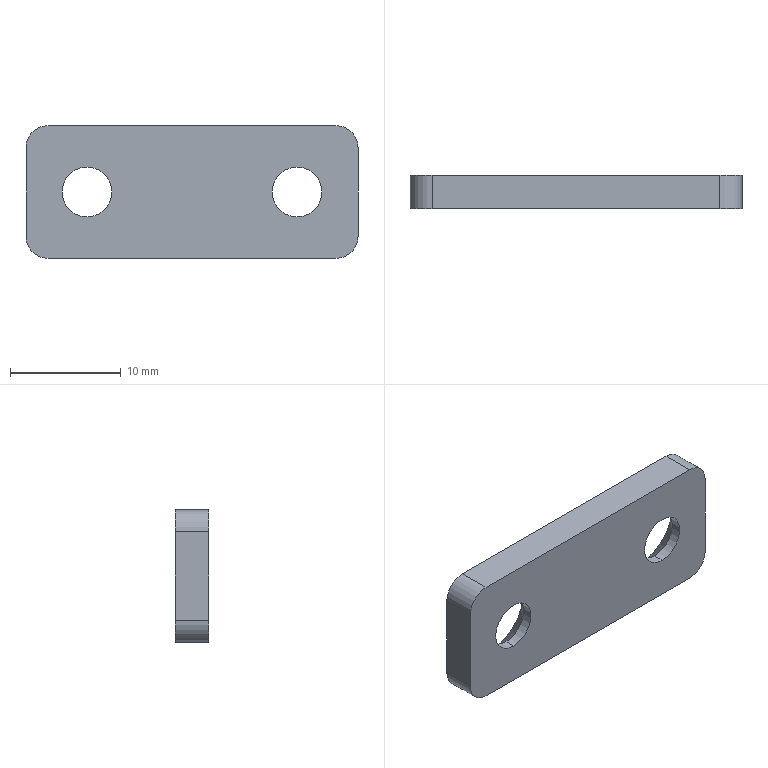Part | STEP file | 03-04 cutter pad block press plate | 1 solid | 18 faces | box 30 x 3 x 12 mm | volume 896.818 mm3 | cylinder 8 | plane 6 | cone 4 | commonest cylinder face diameters 4 x4 4.5 x4
STEP:
#1=CARTESIAN_POINT('',(-9.496,0.95,-2.25));
#2=VERTEX_POINT('',#1);
#3=CARTESIAN_POINT('',(-9.496,0.95,2.25));
#4=VERTEX_POINT('',#3);
#5=CARTESIAN_POINT('',(-9.496,0.95,0.));
#6=DIRECTION('',(0.,1.,0.));
#7=DIRECTION('',(0.,0.,1.));
#8=AXIS2_PLACEMENT_3D('',#5,#6,#7);
#9=CIRCLE('',#8,2.25);
#10=EDGE_CURVE('',#2,#4,#9,.T.);
#11=ORIENTED_EDGE('',*,*,#10,.F.);
#12=CARTESIAN_POINT('',(-9.496,3.,-4.3));
#13=VERTEX_POINT('',#12);
#14=CARTESIAN_POINT('',(-9.496,3.,-4.3));
#15=DIRECTION('',(0.,0.7071,-0.7071));
#16=VECTOR('',#15,1000.);
#17=LINE('',#14,#16);
#18=EDGE_CURVE('',#2,#13,#17,.T.);
#19=ORIENTED_EDGE('',*,*,#18,.T.);
#20=CARTESIAN_POINT('',(-9.496,3.,4.3));
#21=VERTEX_POINT('',#20);
#22=CARTESIAN_POINT('',(-9.496,3.,0.));
#23=DIRECTION('',(0.,1.,0.));
#24=DIRECTION('',(0.,0.,1.));
#25=AXIS2_PLACEMENT_3D('',#22,#23,#24);
#26=CIRCLE('',#25,4.3);
#27=EDGE_CURVE('',#13,#21,#26,.T.);
#28=ORIENTED_EDGE('',*,*,#27,.T.);
#29=CARTESIAN_POINT('',(-9.496,3.,4.3));
#30=DIRECTION('',(0.,0.7071,0.7071));
#31=VECTOR('',#30,1000.);
#32=LINE('',#29,#31);
#33=EDGE_CURVE('',#4,#21,#32,.T.);
#34=ORIENTED_EDGE('',*,*,#33,.F.);
#35=EDGE_LOOP('',(#11,#19,#28,#34));
#36=FACE_OUTER_BOUND('',#35,.T.);
#37=CARTESIAN_POINT('',(-9.496,3.,0.));
#38=DIRECTION('',(0.,1.,0.));
#39=DIRECTION('',(0.,0.,1.));
#40=AXIS2_PLACEMENT_3D('',#37,#38,#39);
#41=CONICAL_SURFACE('',#40,4.3,0.7854);
#42=ADVANCED_FACE('',(#36),#41,.F.);
#43=CARTESIAN_POINT('',(-9.496,0.,-2.25));
#44=VERTEX_POINT('',#43);
#45=CARTESIAN_POINT('',(-9.496,0.,2.25));
#46=VERTEX_POINT('',#45);
#47=CARTESIAN_POINT('',(-9.496,0.,0.));
#48=DIRECTION('',(0.,1.,0.));
#49=DIRECTION('',(0.,0.,1.));
#50=AXIS2_PLACEMENT_3D('',#47,#48,#49);
#51=CIRCLE('',#50,2.25);
#52=EDGE_CURVE('',#44,#46,#51,.T.);
#53=ORIENTED_EDGE('',*,*,#52,.F.);
#54=CARTESIAN_POINT('',(-9.496,3.,-2.25));
#55=DIRECTION('',(0.,1.,0.));
#56=VECTOR('',#55,1000.);
#57=LINE('',#54,#56);
#58=EDGE_CURVE('',#44,#2,#57,.T.);
#59=ORIENTED_EDGE('',*,*,#58,.T.);
#60=ORIENTED_EDGE('',*,*,#10,.T.);
#61=CARTESIAN_POINT('',(-9.496,3.,2.25));
#62=DIRECTION('',(0.,1.,0.));
#63=VECTOR('',#62,1000.);
#64=LINE('',#61,#63);
#65=EDGE_CURVE('',#46,#4,#64,.T.);
#66=ORIENTED_EDGE('',*,*,#65,.F.);
#67=EDGE_LOOP('',(#53,#59,#60,#66));
#68=FACE_OUTER_BOUND('',#67,.T.);
#69=CARTESIAN_POINT('',(-9.496,3.,0.));
#70=DIRECTION('',(0.,1.,0.));
#71=DIRECTION('',(0.,0.,1.));
#72=AXIS2_PLACEMENT_3D('',#69,#70,#71);
#73=CYLINDRICAL_SURFACE('',#72,2.25);
#74=ADVANCED_FACE('',(#68),#73,.F.);
#75=CARTESIAN_POINT('',(9.5,0.95,-2.25));
#76=VERTEX_POINT('',#75);
#77=CARTESIAN_POINT('',(9.5,0.95,2.25));
#78=VERTEX_POINT('',#77);
#79=CARTESIAN_POINT('',(9.5,0.95,0.));
#80=DIRECTION('',(0.,1.,0.));
#81=DIRECTION('',(0.,0.,1.));
#82=AXIS2_PLACEMENT_3D('',#79,#80,#81);
#83=CIRCLE('',#82,2.25);
#84=EDGE_CURVE('',#76,#78,#83,.T.);
#85=ORIENTED_EDGE('',*,*,#84,.F.);
#86=CARTESIAN_POINT('',(9.5,3.,-4.3));
#87=VERTEX_POINT('',#86);
#88=CARTESIAN_POINT('',(9.5,3.,-4.3));
#89=DIRECTION('',(0.,0.7071,-0.7071));
#90=VECTOR('',#89,1000.);
#91=LINE('',#88,#90);
#92=EDGE_CURVE('',#76,#87,#91,.T.);
#93=ORIENTED_EDGE('',*,*,#92,.T.);
#94=CARTESIAN_POINT('',(9.5,3.,4.3));
#95=VERTEX_POINT('',#94);
#96=CARTESIAN_POINT('',(9.5,3.,0.));
#97=DIRECTION('',(0.,1.,0.));
#98=DIRECTION('',(0.,0.,1.));
#99=AXIS2_PLACEMENT_3D('',#96,#97,#98);
#100=CIRCLE('',#99,4.3);
#101=EDGE_CURVE('',#87,#95,#100,.T.);
#102=ORIENTED_EDGE('',*,*,#101,.T.);
#103=CARTESIAN_POINT('',(9.5,3.,4.3));
#104=DIRECTION('',(0.,0.7071,0.7071));
#105=VECTOR('',#104,1000.);
#106=LINE('',#103,#105);
#107=EDGE_CURVE('',#78,#95,#106,.T.);
#108=ORIENTED_EDGE('',*,*,#107,.F.);
#109=EDGE_LOOP('',(#85,#93,#102,#108));
#110=FACE_OUTER_BOUND('',#109,.T.);
#111=CARTESIAN_POINT('',(9.5,3.,0.));
#112=DIRECTION('',(0.,1.,0.));
#113=DIRECTION('',(0.,0.,1.));
#114=AXIS2_PLACEMENT_3D('',#111,#112,#113);
#115=CONICAL_SURFACE('',#114,4.3,0.7854);
#116=ADVANCED_FACE('',(#110),#115,.F.);
#117=CARTESIAN_POINT('',(9.5,0.,-2.25));
#118=VERTEX_POINT('',#117);
#119=CARTESIAN_POINT('',(9.5,0.,2.25));
#120=VERTEX_POINT('',#119);
#121=CARTESIAN_POINT('',(9.5,0.,0.));
#122=DIRECTION('',(0.,1.,0.));
#123=DIRECTION('',(0.,0.,1.));
#124=AXIS2_PLACEMENT_3D('',#121,#122,#123);
#125=CIRCLE('',#124,2.25);
#126=EDGE_CURVE('',#118,#120,#125,.T.);
#127=ORIENTED_EDGE('',*,*,#126,.F.);
#128=CARTESIAN_POINT('',(9.5,3.,-2.25));
#129=DIRECTION('',(0.,1.,0.));
#130=VECTOR('',#129,1000.);
#131=LINE('',#128,#130);
#132=EDGE_CURVE('',#118,#76,#131,.T.);
#133=ORIENTED_EDGE('',*,*,#132,.T.);
#134=ORIENTED_EDGE('',*,*,#84,.T.);
#135=CARTESIAN_POINT('',(9.5,3.,2.25));
#136=DIRECTION('',(0.,1.,0.));
#137=VECTOR('',#136,1000.);
#138=LINE('',#135,#137);
#139=EDGE_CURVE('',#120,#78,#138,.T.);
#140=ORIENTED_EDGE('',*,*,#139,.F.);
#141=EDGE_LOOP('',(#127,#133,#134,#140));
#142=FACE_OUTER_BOUND('',#141,.T.);
#143=CARTESIAN_POINT('',(9.5,3.,0.));
#144=DIRECTION('',(0.,1.,0.));
#145=DIRECTION('',(0.,0.,1.));
#146=AXIS2_PLACEMENT_3D('',#143,#144,#145);
#147=CYLINDRICAL_SURFACE('',#146,2.25);
#148=ADVANCED_FACE('',(#142),#147,.F.);
#149=CARTESIAN_POINT('',(15.,0.,4.));
#150=VERTEX_POINT('',#149);
#151=CARTESIAN_POINT('',(15.,0.,-4.));
#152=VERTEX_POINT('',#151);
#153=CARTESIAN_POINT('',(15.,0.,-6.));
#154=DIRECTION('',(0.,0.,-1.));
#155=VECTOR('',#154,1000.);
#156=LINE('',#153,#155);
#157=EDGE_CURVE('',#150,#152,#156,.T.);
#158=ORIENTED_EDGE('',*,*,#157,.T.);
#159=CARTESIAN_POINT('',(15.,3.,-4.));
#160=VERTEX_POINT('',#159);
#161=CARTESIAN_POINT('',(15.,3.,-4.));
#162=DIRECTION('',(0.,1.,0.));
#163=VECTOR('',#162,1000.);
#164=LINE('',#161,#163);
#165=EDGE_CURVE('',#152,#160,#164,.T.);
#166=ORIENTED_EDGE('',*,*,#165,.T.);
#167=CARTESIAN_POINT('',(15.,3.,4.));
#168=VERTEX_POINT('',#167);
#169=CARTESIAN_POINT('',(15.,3.,-6.));
#170=DIRECTION('',(0.,0.,-1.));
#171=VECTOR('',#170,1000.);
#172=LINE('',#169,#171);
#173=EDGE_CURVE('',#168,#160,#172,.T.);
#174=ORIENTED_EDGE('',*,*,#173,.F.);
#175=CARTESIAN_POINT('',(15.,3.,4.));
#176=DIRECTION('',(0.,-1.,0.));
#177=VECTOR('',#176,1000.);
#178=LINE('',#175,#177);
#179=EDGE_CURVE('',#168,#150,#178,.T.);
#180=ORIENTED_EDGE('',*,*,#179,.T.);
#181=EDGE_LOOP('',(#158,#166,#174,#180));
#182=FACE_OUTER_BOUND('',#181,.T.);
#183=CARTESIAN_POINT('',(15.,3.,-6.));
#184=DIRECTION('',(-1.,0.,0.));
#185=DIRECTION('',(0.,0.,1.));
#186=AXIS2_PLACEMENT_3D('',#183,#184,#185);
#187=PLANE('',#186);
#188=ADVANCED_FACE('',(#182),#187,.F.);
#189=CARTESIAN_POINT('',(13.,3.,-6.));
#190=VERTEX_POINT('',#189);
#191=CARTESIAN_POINT('',(-13.,3.,-6.));
#192=VERTEX_POINT('',#191);
#193=CARTESIAN_POINT('',(-15.,3.,-6.));
#194=DIRECTION('',(-1.,0.,0.));
#195=VECTOR('',#194,1000.);
#196=LINE('',#193,#195);
#197=EDGE_CURVE('',#190,#192,#196,.T.);
#198=ORIENTED_EDGE('',*,*,#197,.F.);
#199=CARTESIAN_POINT('',(13.,0.,-6.));
#200=VERTEX_POINT('',#199);
#201=CARTESIAN_POINT('',(13.,3.,-6.));
#202=DIRECTION('',(0.,-1.,0.));
#203=VECTOR('',#202,1000.);
#204=LINE('',#201,#203);
#205=EDGE_CURVE('',#190,#200,#204,.T.);
#206=ORIENTED_EDGE('',*,*,#205,.T.);
#207=CARTESIAN_POINT('',(-13.,0.,-6.));
#208=VERTEX_POINT('',#207);
#209=CARTESIAN_POINT('',(-15.,0.,-6.));
#210=DIRECTION('',(-1.,0.,0.));
#211=VECTOR('',#210,1000.);
#212=LINE('',#209,#211);
#213=EDGE_CURVE('',#200,#208,#212,.T.);
#214=ORIENTED_EDGE('',*,*,#213,.T.);
#215=CARTESIAN_POINT('',(-13.,3.,-6.));
#216=DIRECTION('',(0.,1.,0.));
#217=VECTOR('',#216,1000.);
#218=LINE('',#215,#217);
#219=EDGE_CURVE('',#208,#192,#218,.T.);
#220=ORIENTED_EDGE('',*,*,#219,.T.);
#221=EDGE_LOOP('',(#198,#206,#214,#220));
#222=FACE_OUTER_BOUND('',#221,.T.);
#223=CARTESIAN_POINT('',(-15.,3.,-6.));
#224=DIRECTION('',(0.,0.,1.));
#225=DIRECTION('',(1.,0.,0.));
#226=AXIS2_PLACEMENT_3D('',#223,#224,#225);
#227=PLANE('',#226);
#228=ADVANCED_FACE('',(#222),#227,.F.);
#229=CARTESIAN_POINT('',(-15.,0.,-4.));
#230=VERTEX_POINT('',#229);
#231=CARTESIAN_POINT('',(-15.,0.,4.));
#232=VERTEX_POINT('',#231);
#233=CARTESIAN_POINT('',(-15.,0.,-6.));
#234=DIRECTION('',(0.,0.,1.));
#235=VECTOR('',#234,1000.);
#236=LINE('',#233,#235);
#237=EDGE_CURVE('',#230,#232,#236,.T.);
#238=ORIENTED_EDGE('',*,*,#237,.T.);
#239=CARTESIAN_POINT('',(-15.,3.,4.));
#240=VERTEX_POINT('',#239);
#241=CARTESIAN_POINT('',(-15.,3.,4.));
#242=DIRECTION('',(0.,1.,0.));
#243=VECTOR('',#242,1000.);
#244=LINE('',#241,#243);
#245=EDGE_CURVE('',#232,#240,#244,.T.);
#246=ORIENTED_EDGE('',*,*,#245,.T.);
#247=CARTESIAN_POINT('',(-15.,3.,-4.));
#248=VERTEX_POINT('',#247);
#249=CARTESIAN_POINT('',(-15.,3.,-6.));
#250=DIRECTION('',(0.,0.,1.));
#251=VECTOR('',#250,1000.);
#252=LINE('',#249,#251);
#253=EDGE_CURVE('',#248,#240,#252,.T.);
#254=ORIENTED_EDGE('',*,*,#253,.F.);
#255=CARTESIAN_POINT('',(-15.,3.,-4.));
#256=DIRECTION('',(0.,-1.,0.));
#257=VECTOR('',#256,1000.);
#258=LINE('',#255,#257);
#259=EDGE_CURVE('',#248,#230,#258,.T.);
#260=ORIENTED_EDGE('',*,*,#259,.T.);
#261=EDGE_LOOP('',(#238,#246,#254,#260));
#262=FACE_OUTER_BOUND('',#261,.T.);
#263=CARTESIAN_POINT('',(-15.,3.,-6.));
#264=DIRECTION('',(1.,0.,0.));
#265=DIRECTION('',(0.,0.,-1.));
#266=AXIS2_PLACEMENT_3D('',#263,#264,#265);
#267=PLANE('',#266);
#268=ADVANCED_FACE('',(#262),#267,.F.);
#269=CARTESIAN_POINT('',(-13.,0.,6.));
#270=VERTEX_POINT('',#269);
#271=CARTESIAN_POINT('',(13.,0.,6.));
#272=VERTEX_POINT('',#271);
#273=CARTESIAN_POINT('',(-15.,0.,6.));
#274=DIRECTION('',(1.,0.,0.));
#275=VECTOR('',#274,1000.);
#276=LINE('',#273,#275);
#277=EDGE_CURVE('',#270,#272,#276,.T.);
#278=ORIENTED_EDGE('',*,*,#277,.T.);
#279=CARTESIAN_POINT('',(13.,3.,6.));
#280=VERTEX_POINT('',#279);
#281=CARTESIAN_POINT('',(13.,3.,6.));
#282=DIRECTION('',(0.,1.,0.));
#283=VECTOR('',#282,1000.);
#284=LINE('',#281,#283);
#285=EDGE_CURVE('',#272,#280,#284,.T.);
#286=ORIENTED_EDGE('',*,*,#285,.T.);
#287=CARTESIAN_POINT('',(-13.,3.,6.));
#288=VERTEX_POINT('',#287);
#289=CARTESIAN_POINT('',(-15.,3.,6.));
#290=DIRECTION('',(1.,0.,0.));
#291=VECTOR('',#290,1000.);
#292=LINE('',#289,#291);
#293=EDGE_CURVE('',#288,#280,#292,.T.);
#294=ORIENTED_EDGE('',*,*,#293,.F.);
#295=CARTESIAN_POINT('',(-13.,3.,6.));
#296=DIRECTION('',(0.,-1.,0.));
#297=VECTOR('',#296,1000.);
#298=LINE('',#295,#297);
#299=EDGE_CURVE('',#288,#270,#298,.T.);
#300=ORIENTED_EDGE('',*,*,#299,.T.);
#301=EDGE_LOOP('',(#278,#286,#294,#300));
#302=FACE_OUTER_BOUND('',#301,.T.);
#303=CARTESIAN_POINT('',(-15.,3.,6.));
#304=DIRECTION('',(0.,0.,-1.));
#305=DIRECTION('',(-1.,0.,0.));
#306=AXIS2_PLACEMENT_3D('',#303,#304,#305);
#307=PLANE('',#306);
#308=ADVANCED_FACE('',(#302),#307,.F.);
#309=CARTESIAN_POINT('',(-9.496,3.,0.));
#310=DIRECTION('',(0.,1.,0.));
#311=DIRECTION('',(0.,0.,1.));
#312=AXIS2_PLACEMENT_3D('',#309,#310,#311);
#313=CIRCLE('',#312,4.3);
#314=EDGE_CURVE('',#21,#13,#313,.T.);
#315=ORIENTED_EDGE('',*,*,#314,.F.);
#316=ORIENTED_EDGE('',*,*,#27,.F.);
#317=EDGE_LOOP('',(#315,#316));
#318=FACE_BOUND('',#317,.T.);
#319=CARTESIAN_POINT('',(9.5,3.,0.));
#320=DIRECTION('',(0.,1.,0.));
#321=DIRECTION('',(0.,0.,1.));
#322=AXIS2_PLACEMENT_3D('',#319,#320,#321);
#323=CIRCLE('',#322,4.3);
#324=EDGE_CURVE('',#95,#87,#323,.T.);
#325=ORIENTED_EDGE('',*,*,#324,.F.);
#326=ORIENTED_EDGE('',*,*,#101,.F.);
#327=EDGE_LOOP('',(#325,#326));
#328=FACE_BOUND('',#327,.T.);
#329=ORIENTED_EDGE('',*,*,#173,.T.);
#330=CARTESIAN_POINT('',(13.,3.,-4.));
#331=DIRECTION('',(0.,1.,0.));
#332=DIRECTION('',(0.,0.,1.));
#333=AXIS2_PLACEMENT_3D('',#330,#331,#332);
#334=CIRCLE('',#333,2.);
#335=EDGE_CURVE('',#160,#190,#334,.T.);
#336=ORIENTED_EDGE('',*,*,#335,.T.);
#337=ORIENTED_EDGE('',*,*,#197,.T.);
#338=CARTESIAN_POINT('',(-13.,3.,-4.));
#339=DIRECTION('',(0.,1.,0.));
#340=DIRECTION('',(0.,0.,1.));
#341=AXIS2_PLACEMENT_3D('',#338,#339,#340);
#342=CIRCLE('',#341,2.);
#343=EDGE_CURVE('',#192,#248,#342,.T.);
#344=ORIENTED_EDGE('',*,*,#343,.T.);
#345=ORIENTED_EDGE('',*,*,#253,.T.);
#346=CARTESIAN_POINT('',(-13.,3.,4.));
#347=DIRECTION('',(0.,1.,0.));
#348=DIRECTION('',(0.,0.,1.));
#349=AXIS2_PLACEMENT_3D('',#346,#347,#348);
#350=CIRCLE('',#349,2.);
#351=EDGE_CURVE('',#240,#288,#350,.T.);
#352=ORIENTED_EDGE('',*,*,#351,.T.);
#353=ORIENTED_EDGE('',*,*,#293,.T.);
#354=CARTESIAN_POINT('',(13.,3.,4.));
#355=DIRECTION('',(0.,1.,0.));
#356=DIRECTION('',(0.,0.,1.));
#357=AXIS2_PLACEMENT_3D('',#354,#355,#356);
#358=CIRCLE('',#357,2.);
#359=EDGE_CURVE('',#280,#168,#358,.T.);
#360=ORIENTED_EDGE('',*,*,#359,.T.);
#361=EDGE_LOOP('',(#329,#336,#337,#344,#345,#352,#353,#360));
#362=FACE_OUTER_BOUND('',#361,.T.);
#363=CARTESIAN_POINT('',(15.,3.,6.));
#364=DIRECTION('',(0.,1.,0.));
#365=DIRECTION('',(0.,0.,1.));
#366=AXIS2_PLACEMENT_3D('',#363,#364,#365);
#367=PLANE('',#366);
#368=ADVANCED_FACE('',(#318,#328,#362),#367,.T.);
#369=CARTESIAN_POINT('',(-9.496,0.,0.));
#370=DIRECTION('',(0.,1.,0.));
#371=DIRECTION('',(0.,0.,1.));
#372=AXIS2_PLACEMENT_3D('',#369,#370,#371);
#373=CIRCLE('',#372,2.25);
#374=EDGE_CURVE('',#46,#44,#373,.T.);
#375=ORIENTED_EDGE('',*,*,#374,.T.);
#376=ORIENTED_EDGE('',*,*,#52,.T.);
#377=EDGE_LOOP('',(#375,#376));
#378=FACE_BOUND('',#377,.T.);
#379=CARTESIAN_POINT('',(9.5,0.,0.));
#380=DIRECTION('',(0.,1.,0.));
#381=DIRECTION('',(0.,0.,1.));
#382=AXIS2_PLACEMENT_3D('',#379,#380,#381);
#383=CIRCLE('',#382,2.25);
#384=EDGE_CURVE('',#120,#118,#383,.T.);
#385=ORIENTED_EDGE('',*,*,#384,.T.);
#386=ORIENTED_EDGE('',*,*,#126,.T.);
#387=EDGE_LOOP('',(#385,#386));
#388=FACE_BOUND('',#387,.T.);
#389=ORIENTED_EDGE('',*,*,#213,.F.);
#390=CARTESIAN_POINT('',(13.,0.,-4.));
#391=DIRECTION('',(0.,-1.,0.));
#392=DIRECTION('',(0.,0.,1.));
#393=AXIS2_PLACEMENT_3D('',#390,#391,#392);
#394=CIRCLE('',#393,2.);
#395=EDGE_CURVE('',#200,#152,#394,.T.);
#396=ORIENTED_EDGE('',*,*,#395,.T.);
#397=ORIENTED_EDGE('',*,*,#157,.F.);
#398=CARTESIAN_POINT('',(13.,0.,4.));
#399=DIRECTION('',(0.,-1.,0.));
#400=DIRECTION('',(0.,0.,1.));
#401=AXIS2_PLACEMENT_3D('',#398,#399,#400);
#402=CIRCLE('',#401,2.);
#403=EDGE_CURVE('',#150,#272,#402,.T.);
#404=ORIENTED_EDGE('',*,*,#403,.T.);
#405=ORIENTED_EDGE('',*,*,#277,.F.);
#406=CARTESIAN_POINT('',(-13.,0.,4.));
#407=DIRECTION('',(0.,-1.,0.));
#408=DIRECTION('',(0.,0.,1.));
#409=AXIS2_PLACEMENT_3D('',#406,#407,#408);
#410=CIRCLE('',#409,2.);
#411=EDGE_CURVE('',#270,#232,#410,.T.);
#412=ORIENTED_EDGE('',*,*,#411,.T.);
#413=ORIENTED_EDGE('',*,*,#237,.F.);
#414=CARTESIAN_POINT('',(-13.,0.,-4.));
#415=DIRECTION('',(0.,-1.,0.));
#416=DIRECTION('',(0.,0.,1.));
#417=AXIS2_PLACEMENT_3D('',#414,#415,#416);
#418=CIRCLE('',#417,2.);
#419=EDGE_CURVE('',#230,#208,#418,.T.);
#420=ORIENTED_EDGE('',*,*,#419,.T.);
#421=EDGE_LOOP('',(#389,#396,#397,#404,#405,#412,#413,#420));
#422=FACE_OUTER_BOUND('',#421,.T.);
#423=CARTESIAN_POINT('',(15.,0.,6.));
#424=DIRECTION('',(0.,1.,0.));
#425=DIRECTION('',(0.,0.,1.));
#426=AXIS2_PLACEMENT_3D('',#423,#424,#425);
#427=PLANE('',#426);
#428=ADVANCED_FACE('',(#378,#388,#422),#427,.F.);
#429=ORIENTED_EDGE('',*,*,#335,.F.);
#430=ORIENTED_EDGE('',*,*,#165,.F.);
#431=ORIENTED_EDGE('',*,*,#395,.F.);
#432=ORIENTED_EDGE('',*,*,#205,.F.);
#433=EDGE_LOOP('',(#429,#430,#431,#432));
#434=FACE_OUTER_BOUND('',#433,.T.);
#435=CARTESIAN_POINT('',(13.,3.,-4.));
#436=DIRECTION('',(0.,-1.,0.));
#437=DIRECTION('',(0.,0.,-1.));
#438=AXIS2_PLACEMENT_3D('',#435,#436,#437);
#439=CYLINDRICAL_SURFACE('',#438,2.);
#440=ADVANCED_FACE('',(#434),#439,.T.);
#441=ORIENTED_EDGE('',*,*,#359,.F.);
#442=ORIENTED_EDGE('',*,*,#285,.F.);
#443=ORIENTED_EDGE('',*,*,#403,.F.);
#444=ORIENTED_EDGE('',*,*,#179,.F.);
#445=EDGE_LOOP('',(#441,#442,#443,#444));
#446=FACE_OUTER_BOUND('',#445,.T.);
#447=CARTESIAN_POINT('',(13.,3.,4.));
#448=DIRECTION('',(0.,-1.,0.));
#449=DIRECTION('',(0.,0.,-1.));
#450=AXIS2_PLACEMENT_3D('',#447,#448,#449);
#451=CYLINDRICAL_SURFACE('',#450,2.);
#452=ADVANCED_FACE('',(#446),#451,.T.);
#453=ORIENTED_EDGE('',*,*,#351,.F.);
#454=ORIENTED_EDGE('',*,*,#245,.F.);
#455=ORIENTED_EDGE('',*,*,#411,.F.);
#456=ORIENTED_EDGE('',*,*,#299,.F.);
#457=EDGE_LOOP('',(#453,#454,#455,#456));
#458=FACE_OUTER_BOUND('',#457,.T.);
#459=CARTESIAN_POINT('',(-13.,3.,4.));
#460=DIRECTION('',(0.,-1.,0.));
#461=DIRECTION('',(0.,0.,-1.));
#462=AXIS2_PLACEMENT_3D('',#459,#460,#461);
#463=CYLINDRICAL_SURFACE('',#462,2.);
#464=ADVANCED_FACE('',(#458),#463,.T.);
#465=ORIENTED_EDGE('',*,*,#343,.F.);
#466=ORIENTED_EDGE('',*,*,#219,.F.);
#467=ORIENTED_EDGE('',*,*,#419,.F.);
#468=ORIENTED_EDGE('',*,*,#259,.F.);
#469=EDGE_LOOP('',(#465,#466,#467,#468));
#470=FACE_OUTER_BOUND('',#469,.T.);
#471=CARTESIAN_POINT('',(-13.,3.,-4.));
#472=DIRECTION('',(0.,-1.,0.));
#473=DIRECTION('',(0.,0.,-1.));
#474=AXIS2_PLACEMENT_3D('',#471,#472,#473);
#475=CYLINDRICAL_SURFACE('',#474,2.);
#476=ADVANCED_FACE('',(#470),#475,.T.);
#477=ORIENTED_EDGE('',*,*,#132,.F.);
#478=ORIENTED_EDGE('',*,*,#384,.F.);
#479=ORIENTED_EDGE('',*,*,#139,.T.);
#480=CARTESIAN_POINT('',(9.5,0.95,0.));
#481=DIRECTION('',(0.,1.,0.));
#482=DIRECTION('',(0.,0.,1.));
#483=AXIS2_PLACEMENT_3D('',#480,#481,#482);
#484=CIRCLE('',#483,2.25);
#485=EDGE_CURVE('',#78,#76,#484,.T.);
#486=ORIENTED_EDGE('',*,*,#485,.T.);
#487=EDGE_LOOP('',(#477,#478,#479,#486));
#488=FACE_OUTER_BOUND('',#487,.T.);
#489=CARTESIAN_POINT('',(9.5,3.,0.));
#490=DIRECTION('',(0.,1.,0.));
#491=DIRECTION('',(0.,0.,1.));
#492=AXIS2_PLACEMENT_3D('',#489,#490,#491);
#493=CYLINDRICAL_SURFACE('',#492,2.25);
#494=ADVANCED_FACE('',(#488),#493,.F.);
#495=ORIENTED_EDGE('',*,*,#92,.F.);
#496=ORIENTED_EDGE('',*,*,#485,.F.);
#497=ORIENTED_EDGE('',*,*,#107,.T.);
#498=ORIENTED_EDGE('',*,*,#324,.T.);
#499=EDGE_LOOP('',(#495,#496,#497,#498));
#500=FACE_OUTER_BOUND('',#499,.T.);
#501=CARTESIAN_POINT('',(9.5,3.,0.));
#502=DIRECTION('',(0.,1.,0.));
#503=DIRECTION('',(0.,0.,1.));
#504=AXIS2_PLACEMENT_3D('',#501,#502,#503);
#505=CONICAL_SURFACE('',#504,4.3,0.7854);
#506=ADVANCED_FACE('',(#500),#505,.F.);
#507=ORIENTED_EDGE('',*,*,#58,.F.);
#508=ORIENTED_EDGE('',*,*,#374,.F.);
#509=ORIENTED_EDGE('',*,*,#65,.T.);
#510=CARTESIAN_POINT('',(-9.496,0.95,0.));
#511=DIRECTION('',(0.,1.,0.));
#512=DIRECTION('',(0.,0.,1.));
#513=AXIS2_PLACEMENT_3D('',#510,#511,#512);
#514=CIRCLE('',#513,2.25);
#515=EDGE_CURVE('',#4,#2,#514,.T.);
#516=ORIENTED_EDGE('',*,*,#515,.T.);
#517=EDGE_LOOP('',(#507,#508,#509,#516));
#518=FACE_OUTER_BOUND('',#517,.T.);
#519=CARTESIAN_POINT('',(-9.496,3.,0.));
#520=DIRECTION('',(0.,1.,0.));
#521=DIRECTION('',(0.,0.,1.));
#522=AXIS2_PLACEMENT_3D('',#519,#520,#521);
#523=CYLINDRICAL_SURFACE('',#522,2.25);
#524=ADVANCED_FACE('',(#518),#523,.F.);
#525=ORIENTED_EDGE('',*,*,#18,.F.);
#526=ORIENTED_EDGE('',*,*,#515,.F.);
#527=ORIENTED_EDGE('',*,*,#33,.T.);
#528=ORIENTED_EDGE('',*,*,#314,.T.);
#529=EDGE_LOOP('',(#525,#526,#527,#528));
#530=FACE_OUTER_BOUND('',#529,.T.);
#531=CARTESIAN_POINT('',(-9.496,3.,0.));
#532=DIRECTION('',(0.,1.,0.));
#533=DIRECTION('',(0.,0.,1.));
#534=AXIS2_PLACEMENT_3D('',#531,#532,#533);
#535=CONICAL_SURFACE('',#534,4.3,0.7854);
#536=ADVANCED_FACE('',(#530),#535,.F.);
#537=CLOSED_SHELL('',(#42,#74,#116,#148,#188,#228,#268,#308,#368,#428,#440,#452,#464,#476,#494,#506,#524,#536));
#538=MANIFOLD_SOLID_BREP('',#537);
#539=CARTESIAN_POINT('',(0.,0.,0.));
#540=DIRECTION('',(0.,0.,1.));
#541=DIRECTION('',(1.,0.,0.));
#542=AXIS2_PLACEMENT_3D('',#539,#540,#541);
#543=(LENGTH_UNIT()NAMED_UNIT(*)SI_UNIT(.MILLI.,.METRE.));
#544=UNCERTAINTY_MEASURE_WITH_UNIT(LENGTH_MEASURE(0.00001),#543,'','');
#545=(NAMED_UNIT(*)PLANE_ANGLE_UNIT()SI_UNIT($,.RADIAN.));
#546=(NAMED_UNIT(*)SI_UNIT($,.STERADIAN.)SOLID_ANGLE_UNIT());
#547=(GEOMETRIC_REPRESENTATION_CONTEXT(3)GLOBAL_UNCERTAINTY_ASSIGNED_CONTEXT((#544))GLOBAL_UNIT_ASSIGNED_CONTEXT((#543,#545,#546))REPRESENTATION_CONTEXT('',''));
#548=ADVANCED_BREP_SHAPE_REPRESENTATION('',(#538,#542),#547);